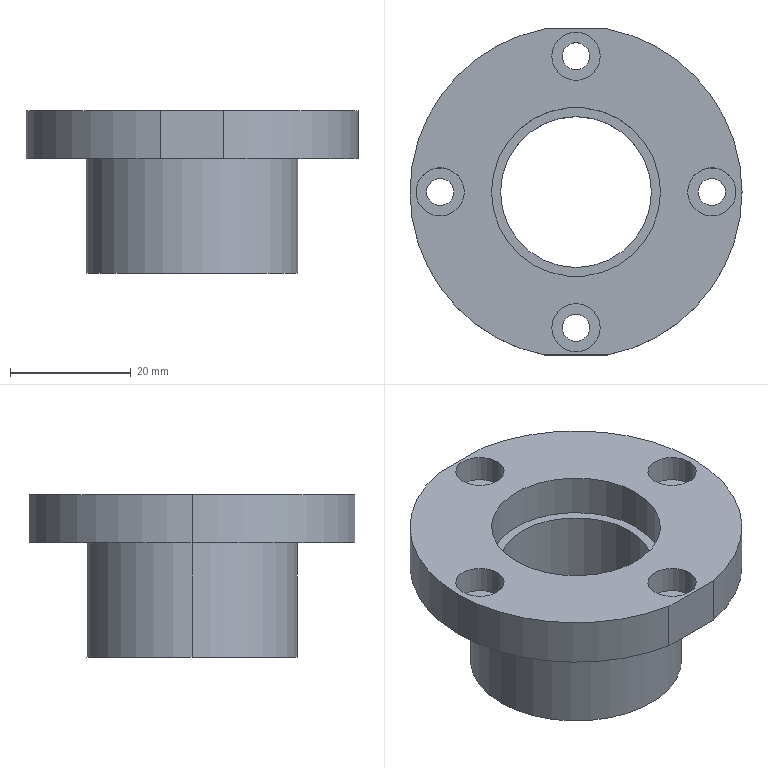Part | STEP file | 11-FG-E03611 | 1 solid | 38 faces | box 55 x 54 x 27 mm | volume 21102 mm3 | cylinder 27 | plane 11 | commonest cylinder face diameters 4.5 x8 8 x8 28 x4 55 x3 25 x2 35 x2
STEP:
#1=CARTESIAN_POINT('',(-26.5,0.,22.5));
#2=VERTEX_POINT('',#1);
#3=CARTESIAN_POINT('',(-18.5,0.,22.5));
#4=VERTEX_POINT('',#3);
#5=CARTESIAN_POINT('',(-22.5,0.,22.5));
#6=DIRECTION('',(0.,0.,1.));
#7=DIRECTION('',(1.,0.,0.));
#8=AXIS2_PLACEMENT_3D('',#5,#6,#7);
#9=CIRCLE('',#8,4.);
#10=EDGE_CURVE('',#2,#4,#9,.T.);
#11=ORIENTED_EDGE('',*,*,#10,.F.);
#12=CARTESIAN_POINT('',(-26.5,0.,27.));
#13=VERTEX_POINT('',#12);
#14=CARTESIAN_POINT('',(-26.5,0.,27.));
#15=DIRECTION('',(0.,0.,1.));
#16=VECTOR('',#15,1000.);
#17=LINE('',#14,#16);
#18=EDGE_CURVE('',#2,#13,#17,.T.);
#19=ORIENTED_EDGE('',*,*,#18,.T.);
#20=CARTESIAN_POINT('',(-18.5,0.,27.));
#21=VERTEX_POINT('',#20);
#22=CARTESIAN_POINT('',(-22.5,0.,27.));
#23=DIRECTION('',(0.,0.,1.));
#24=DIRECTION('',(1.,0.,0.));
#25=AXIS2_PLACEMENT_3D('',#22,#23,#24);
#26=CIRCLE('',#25,4.);
#27=EDGE_CURVE('',#13,#21,#26,.T.);
#28=ORIENTED_EDGE('',*,*,#27,.T.);
#29=CARTESIAN_POINT('',(-18.5,0.,27.));
#30=DIRECTION('',(0.,0.,1.));
#31=VECTOR('',#30,1000.);
#32=LINE('',#29,#31);
#33=EDGE_CURVE('',#4,#21,#32,.T.);
#34=ORIENTED_EDGE('',*,*,#33,.F.);
#35=EDGE_LOOP('',(#11,#19,#28,#34));
#36=FACE_OUTER_BOUND('',#35,.T.);
#37=CARTESIAN_POINT('',(-22.5,0.,27.));
#38=DIRECTION('',(0.,0.,1.));
#39=DIRECTION('',(1.,0.,0.));
#40=AXIS2_PLACEMENT_3D('',#37,#38,#39);
#41=CYLINDRICAL_SURFACE('',#40,4.);
#42=ADVANCED_FACE('',(#36),#41,.F.);
#43=CARTESIAN_POINT('',(-24.75,0.,19.));
#44=VERTEX_POINT('',#43);
#45=CARTESIAN_POINT('',(-20.25,0.,19.));
#46=VERTEX_POINT('',#45);
#47=CARTESIAN_POINT('',(-22.5,0.,19.));
#48=DIRECTION('',(0.,0.,1.));
#49=DIRECTION('',(1.,0.,0.));
#50=AXIS2_PLACEMENT_3D('',#47,#48,#49);
#51=CIRCLE('',#50,2.25);
#52=EDGE_CURVE('',#44,#46,#51,.T.);
#53=ORIENTED_EDGE('',*,*,#52,.F.);
#54=CARTESIAN_POINT('',(-24.75,0.,22.5));
#55=VERTEX_POINT('',#54);
#56=CARTESIAN_POINT('',(-24.75,0.,27.));
#57=DIRECTION('',(0.,0.,1.));
#58=VECTOR('',#57,1000.);
#59=LINE('',#56,#58);
#60=EDGE_CURVE('',#44,#55,#59,.T.);
#61=ORIENTED_EDGE('',*,*,#60,.T.);
#62=CARTESIAN_POINT('',(-20.25,0.,22.5));
#63=VERTEX_POINT('',#62);
#64=CARTESIAN_POINT('',(-22.5,0.,22.5));
#65=DIRECTION('',(0.,0.,1.));
#66=DIRECTION('',(1.,0.,0.));
#67=AXIS2_PLACEMENT_3D('',#64,#65,#66);
#68=CIRCLE('',#67,2.25);
#69=EDGE_CURVE('',#55,#63,#68,.T.);
#70=ORIENTED_EDGE('',*,*,#69,.T.);
#71=CARTESIAN_POINT('',(-20.25,0.,27.));
#72=DIRECTION('',(0.,0.,1.));
#73=VECTOR('',#72,1000.);
#74=LINE('',#71,#73);
#75=EDGE_CURVE('',#46,#63,#74,.T.);
#76=ORIENTED_EDGE('',*,*,#75,.F.);
#77=EDGE_LOOP('',(#53,#61,#70,#76));
#78=FACE_OUTER_BOUND('',#77,.T.);
#79=CARTESIAN_POINT('',(-22.5,0.,27.));
#80=DIRECTION('',(0.,0.,1.));
#81=DIRECTION('',(1.,0.,0.));
#82=AXIS2_PLACEMENT_3D('',#79,#80,#81);
#83=CYLINDRICAL_SURFACE('',#82,2.25);
#84=ADVANCED_FACE('',(#78),#83,.F.);
#85=CARTESIAN_POINT('',(-4.,-22.5,22.5));
#86=VERTEX_POINT('',#85);
#87=CARTESIAN_POINT('',(4.,-22.5,22.5));
#88=VERTEX_POINT('',#87);
#89=CARTESIAN_POINT('',(0.,-22.5,22.5));
#90=DIRECTION('',(0.,0.,1.));
#91=DIRECTION('',(1.,0.,0.));
#92=AXIS2_PLACEMENT_3D('',#89,#90,#91);
#93=CIRCLE('',#92,4.);
#94=EDGE_CURVE('',#86,#88,#93,.T.);
#95=ORIENTED_EDGE('',*,*,#94,.F.);
#96=CARTESIAN_POINT('',(-4.,-22.5,27.));
#97=VERTEX_POINT('',#96);
#98=CARTESIAN_POINT('',(-4.,-22.5,27.));
#99=DIRECTION('',(0.,0.,1.));
#100=VECTOR('',#99,1000.);
#101=LINE('',#98,#100);
#102=EDGE_CURVE('',#86,#97,#101,.T.);
#103=ORIENTED_EDGE('',*,*,#102,.T.);
#104=CARTESIAN_POINT('',(4.,-22.5,27.));
#105=VERTEX_POINT('',#104);
#106=CARTESIAN_POINT('',(0.,-22.5,27.));
#107=DIRECTION('',(0.,0.,1.));
#108=DIRECTION('',(1.,0.,0.));
#109=AXIS2_PLACEMENT_3D('',#106,#107,#108);
#110=CIRCLE('',#109,4.);
#111=EDGE_CURVE('',#97,#105,#110,.T.);
#112=ORIENTED_EDGE('',*,*,#111,.T.);
#113=CARTESIAN_POINT('',(4.,-22.5,27.));
#114=DIRECTION('',(0.,0.,1.));
#115=VECTOR('',#114,1000.);
#116=LINE('',#113,#115);
#117=EDGE_CURVE('',#88,#105,#116,.T.);
#118=ORIENTED_EDGE('',*,*,#117,.F.);
#119=EDGE_LOOP('',(#95,#103,#112,#118));
#120=FACE_OUTER_BOUND('',#119,.T.);
#121=CARTESIAN_POINT('',(0.,-22.5,27.));
#122=DIRECTION('',(0.,0.,1.));
#123=DIRECTION('',(1.,0.,0.));
#124=AXIS2_PLACEMENT_3D('',#121,#122,#123);
#125=CYLINDRICAL_SURFACE('',#124,4.);
#126=ADVANCED_FACE('',(#120),#125,.F.);
#127=CARTESIAN_POINT('',(-2.25,-22.5,19.));
#128=VERTEX_POINT('',#127);
#129=CARTESIAN_POINT('',(2.25,-22.5,19.));
#130=VERTEX_POINT('',#129);
#131=CARTESIAN_POINT('',(0.,-22.5,19.));
#132=DIRECTION('',(0.,0.,1.));
#133=DIRECTION('',(1.,0.,0.));
#134=AXIS2_PLACEMENT_3D('',#131,#132,#133);
#135=CIRCLE('',#134,2.25);
#136=EDGE_CURVE('',#128,#130,#135,.T.);
#137=ORIENTED_EDGE('',*,*,#136,.F.);
#138=CARTESIAN_POINT('',(-2.25,-22.5,22.5));
#139=VERTEX_POINT('',#138);
#140=CARTESIAN_POINT('',(-2.25,-22.5,27.));
#141=DIRECTION('',(0.,0.,1.));
#142=VECTOR('',#141,1000.);
#143=LINE('',#140,#142);
#144=EDGE_CURVE('',#128,#139,#143,.T.);
#145=ORIENTED_EDGE('',*,*,#144,.T.);
#146=CARTESIAN_POINT('',(2.25,-22.5,22.5));
#147=VERTEX_POINT('',#146);
#148=CARTESIAN_POINT('',(0.,-22.5,22.5));
#149=DIRECTION('',(0.,0.,1.));
#150=DIRECTION('',(1.,0.,0.));
#151=AXIS2_PLACEMENT_3D('',#148,#149,#150);
#152=CIRCLE('',#151,2.25);
#153=EDGE_CURVE('',#139,#147,#152,.T.);
#154=ORIENTED_EDGE('',*,*,#153,.T.);
#155=CARTESIAN_POINT('',(2.25,-22.5,27.));
#156=DIRECTION('',(0.,0.,1.));
#157=VECTOR('',#156,1000.);
#158=LINE('',#155,#157);
#159=EDGE_CURVE('',#130,#147,#158,.T.);
#160=ORIENTED_EDGE('',*,*,#159,.F.);
#161=EDGE_LOOP('',(#137,#145,#154,#160));
#162=FACE_OUTER_BOUND('',#161,.T.);
#163=CARTESIAN_POINT('',(0.,-22.5,27.));
#164=DIRECTION('',(0.,0.,1.));
#165=DIRECTION('',(1.,0.,0.));
#166=AXIS2_PLACEMENT_3D('',#163,#164,#165);
#167=CYLINDRICAL_SURFACE('',#166,2.25);
#168=ADVANCED_FACE('',(#162),#167,.F.);
#169=CARTESIAN_POINT('',(18.5,0.,22.5));
#170=VERTEX_POINT('',#169);
#171=CARTESIAN_POINT('',(26.5,0.,22.5));
#172=VERTEX_POINT('',#171);
#173=CARTESIAN_POINT('',(22.5,0.,22.5));
#174=DIRECTION('',(0.,0.,1.));
#175=DIRECTION('',(1.,0.,0.));
#176=AXIS2_PLACEMENT_3D('',#173,#174,#175);
#177=CIRCLE('',#176,4.);
#178=EDGE_CURVE('',#170,#172,#177,.T.);
#179=ORIENTED_EDGE('',*,*,#178,.F.);
#180=CARTESIAN_POINT('',(18.5,0.,27.));
#181=VERTEX_POINT('',#180);
#182=CARTESIAN_POINT('',(18.5,0.,27.));
#183=DIRECTION('',(0.,0.,1.));
#184=VECTOR('',#183,1000.);
#185=LINE('',#182,#184);
#186=EDGE_CURVE('',#170,#181,#185,.T.);
#187=ORIENTED_EDGE('',*,*,#186,.T.);
#188=CARTESIAN_POINT('',(26.5,0.,27.));
#189=VERTEX_POINT('',#188);
#190=CARTESIAN_POINT('',(22.5,0.,27.));
#191=DIRECTION('',(0.,0.,1.));
#192=DIRECTION('',(1.,0.,0.));
#193=AXIS2_PLACEMENT_3D('',#190,#191,#192);
#194=CIRCLE('',#193,4.);
#195=EDGE_CURVE('',#181,#189,#194,.T.);
#196=ORIENTED_EDGE('',*,*,#195,.T.);
#197=CARTESIAN_POINT('',(26.5,0.,27.));
#198=DIRECTION('',(0.,0.,1.));
#199=VECTOR('',#198,1000.);
#200=LINE('',#197,#199);
#201=EDGE_CURVE('',#172,#189,#200,.T.);
#202=ORIENTED_EDGE('',*,*,#201,.F.);
#203=EDGE_LOOP('',(#179,#187,#196,#202));
#204=FACE_OUTER_BOUND('',#203,.T.);
#205=CARTESIAN_POINT('',(22.5,0.,27.));
#206=DIRECTION('',(0.,0.,1.));
#207=DIRECTION('',(1.,0.,0.));
#208=AXIS2_PLACEMENT_3D('',#205,#206,#207);
#209=CYLINDRICAL_SURFACE('',#208,4.);
#210=ADVANCED_FACE('',(#204),#209,.F.);
#211=CARTESIAN_POINT('',(20.25,0.,19.));
#212=VERTEX_POINT('',#211);
#213=CARTESIAN_POINT('',(24.75,0.,19.));
#214=VERTEX_POINT('',#213);
#215=CARTESIAN_POINT('',(22.5,0.,19.));
#216=DIRECTION('',(0.,0.,1.));
#217=DIRECTION('',(1.,0.,0.));
#218=AXIS2_PLACEMENT_3D('',#215,#216,#217);
#219=CIRCLE('',#218,2.25);
#220=EDGE_CURVE('',#212,#214,#219,.T.);
#221=ORIENTED_EDGE('',*,*,#220,.F.);
#222=CARTESIAN_POINT('',(20.25,0.,22.5));
#223=VERTEX_POINT('',#222);
#224=CARTESIAN_POINT('',(20.25,0.,27.));
#225=DIRECTION('',(0.,0.,1.));
#226=VECTOR('',#225,1000.);
#227=LINE('',#224,#226);
#228=EDGE_CURVE('',#212,#223,#227,.T.);
#229=ORIENTED_EDGE('',*,*,#228,.T.);
#230=CARTESIAN_POINT('',(24.75,0.,22.5));
#231=VERTEX_POINT('',#230);
#232=CARTESIAN_POINT('',(22.5,0.,22.5));
#233=DIRECTION('',(0.,0.,1.));
#234=DIRECTION('',(1.,0.,0.));
#235=AXIS2_PLACEMENT_3D('',#232,#233,#234);
#236=CIRCLE('',#235,2.25);
#237=EDGE_CURVE('',#223,#231,#236,.T.);
#238=ORIENTED_EDGE('',*,*,#237,.T.);
#239=CARTESIAN_POINT('',(24.75,0.,27.));
#240=DIRECTION('',(0.,0.,1.));
#241=VECTOR('',#240,1000.);
#242=LINE('',#239,#241);
#243=EDGE_CURVE('',#214,#231,#242,.T.);
#244=ORIENTED_EDGE('',*,*,#243,.F.);
#245=EDGE_LOOP('',(#221,#229,#238,#244));
#246=FACE_OUTER_BOUND('',#245,.T.);
#247=CARTESIAN_POINT('',(22.5,0.,27.));
#248=DIRECTION('',(0.,0.,1.));
#249=DIRECTION('',(1.,0.,0.));
#250=AXIS2_PLACEMENT_3D('',#247,#248,#249);
#251=CYLINDRICAL_SURFACE('',#250,2.25);
#252=ADVANCED_FACE('',(#246),#251,.F.);
#253=CARTESIAN_POINT('',(-4.,22.5,22.5));
#254=VERTEX_POINT('',#253);
#255=CARTESIAN_POINT('',(4.,22.5,22.5));
#256=VERTEX_POINT('',#255);
#257=CARTESIAN_POINT('',(0.,22.5,22.5));
#258=DIRECTION('',(0.,0.,1.));
#259=DIRECTION('',(1.,0.,0.));
#260=AXIS2_PLACEMENT_3D('',#257,#258,#259);
#261=CIRCLE('',#260,4.);
#262=EDGE_CURVE('',#254,#256,#261,.T.);
#263=ORIENTED_EDGE('',*,*,#262,.F.);
#264=CARTESIAN_POINT('',(-4.,22.5,27.));
#265=VERTEX_POINT('',#264);
#266=CARTESIAN_POINT('',(-4.,22.5,27.));
#267=DIRECTION('',(0.,0.,1.));
#268=VECTOR('',#267,1000.);
#269=LINE('',#266,#268);
#270=EDGE_CURVE('',#254,#265,#269,.T.);
#271=ORIENTED_EDGE('',*,*,#270,.T.);
#272=CARTESIAN_POINT('',(4.,22.5,27.));
#273=VERTEX_POINT('',#272);
#274=CARTESIAN_POINT('',(0.,22.5,27.));
#275=DIRECTION('',(0.,0.,1.));
#276=DIRECTION('',(1.,0.,0.));
#277=AXIS2_PLACEMENT_3D('',#274,#275,#276);
#278=CIRCLE('',#277,4.);
#279=EDGE_CURVE('',#265,#273,#278,.T.);
#280=ORIENTED_EDGE('',*,*,#279,.T.);
#281=CARTESIAN_POINT('',(4.,22.5,27.));
#282=DIRECTION('',(0.,0.,1.));
#283=VECTOR('',#282,1000.);
#284=LINE('',#281,#283);
#285=EDGE_CURVE('',#256,#273,#284,.T.);
#286=ORIENTED_EDGE('',*,*,#285,.F.);
#287=EDGE_LOOP('',(#263,#271,#280,#286));
#288=FACE_OUTER_BOUND('',#287,.T.);
#289=CARTESIAN_POINT('',(0.,22.5,27.));
#290=DIRECTION('',(0.,0.,1.));
#291=DIRECTION('',(1.,0.,0.));
#292=AXIS2_PLACEMENT_3D('',#289,#290,#291);
#293=CYLINDRICAL_SURFACE('',#292,4.);
#294=ADVANCED_FACE('',(#288),#293,.F.);
#295=CARTESIAN_POINT('',(-2.25,22.5,19.));
#296=VERTEX_POINT('',#295);
#297=CARTESIAN_POINT('',(2.25,22.5,19.));
#298=VERTEX_POINT('',#297);
#299=CARTESIAN_POINT('',(0.,22.5,19.));
#300=DIRECTION('',(0.,0.,1.));
#301=DIRECTION('',(1.,0.,0.));
#302=AXIS2_PLACEMENT_3D('',#299,#300,#301);
#303=CIRCLE('',#302,2.25);
#304=EDGE_CURVE('',#296,#298,#303,.T.);
#305=ORIENTED_EDGE('',*,*,#304,.F.);
#306=CARTESIAN_POINT('',(-2.25,22.5,22.5));
#307=VERTEX_POINT('',#306);
#308=CARTESIAN_POINT('',(-2.25,22.5,27.));
#309=DIRECTION('',(0.,0.,1.));
#310=VECTOR('',#309,1000.);
#311=LINE('',#308,#310);
#312=EDGE_CURVE('',#296,#307,#311,.T.);
#313=ORIENTED_EDGE('',*,*,#312,.T.);
#314=CARTESIAN_POINT('',(2.25,22.5,22.5));
#315=VERTEX_POINT('',#314);
#316=CARTESIAN_POINT('',(0.,22.5,22.5));
#317=DIRECTION('',(0.,0.,1.));
#318=DIRECTION('',(1.,0.,0.));
#319=AXIS2_PLACEMENT_3D('',#316,#317,#318);
#320=CIRCLE('',#319,2.25);
#321=EDGE_CURVE('',#307,#315,#320,.T.);
#322=ORIENTED_EDGE('',*,*,#321,.T.);
#323=CARTESIAN_POINT('',(2.25,22.5,27.));
#324=DIRECTION('',(0.,0.,1.));
#325=VECTOR('',#324,1000.);
#326=LINE('',#323,#325);
#327=EDGE_CURVE('',#298,#315,#326,.T.);
#328=ORIENTED_EDGE('',*,*,#327,.F.);
#329=EDGE_LOOP('',(#305,#313,#322,#328));
#330=FACE_OUTER_BOUND('',#329,.T.);
#331=CARTESIAN_POINT('',(0.,22.5,27.));
#332=DIRECTION('',(0.,0.,1.));
#333=DIRECTION('',(1.,0.,0.));
#334=AXIS2_PLACEMENT_3D('',#331,#332,#333);
#335=CYLINDRICAL_SURFACE('',#334,2.25);
#336=ADVANCED_FACE('',(#330),#335,.F.);
#337=CARTESIAN_POINT('',(-14.,0.,20.));
#338=VERTEX_POINT('',#337);
#339=CARTESIAN_POINT('',(14.,0.,20.));
#340=VERTEX_POINT('',#339);
#341=CARTESIAN_POINT('',(0.,0.,20.));
#342=DIRECTION('',(0.,0.,1.));
#343=DIRECTION('',(1.,0.,0.));
#344=AXIS2_PLACEMENT_3D('',#341,#342,#343);
#345=CIRCLE('',#344,14.);
#346=EDGE_CURVE('',#338,#340,#345,.T.);
#347=ORIENTED_EDGE('',*,*,#346,.F.);
#348=CARTESIAN_POINT('',(-14.,0.,27.));
#349=VERTEX_POINT('',#348);
#350=CARTESIAN_POINT('',(-14.,0.,20.));
#351=DIRECTION('',(0.,0.,1.));
#352=VECTOR('',#351,1000.);
#353=LINE('',#350,#352);
#354=EDGE_CURVE('',#338,#349,#353,.T.);
#355=ORIENTED_EDGE('',*,*,#354,.T.);
#356=CARTESIAN_POINT('',(14.,0.,27.));
#357=VERTEX_POINT('',#356);
#358=CARTESIAN_POINT('',(0.,0.,27.));
#359=DIRECTION('',(0.,0.,1.));
#360=DIRECTION('',(1.,0.,0.));
#361=AXIS2_PLACEMENT_3D('',#358,#359,#360);
#362=CIRCLE('',#361,14.);
#363=EDGE_CURVE('',#349,#357,#362,.T.);
#364=ORIENTED_EDGE('',*,*,#363,.T.);
#365=CARTESIAN_POINT('',(14.,0.,20.));
#366=DIRECTION('',(0.,0.,1.));
#367=VECTOR('',#366,1000.);
#368=LINE('',#365,#367);
#369=EDGE_CURVE('',#340,#357,#368,.T.);
#370=ORIENTED_EDGE('',*,*,#369,.F.);
#371=EDGE_LOOP('',(#347,#355,#364,#370));
#372=FACE_OUTER_BOUND('',#371,.T.);
#373=CARTESIAN_POINT('',(0.,0.,20.));
#374=DIRECTION('',(0.,0.,1.));
#375=DIRECTION('',(1.,0.,0.));
#376=AXIS2_PLACEMENT_3D('',#373,#374,#375);
#377=CYLINDRICAL_SURFACE('',#376,14.);
#378=ADVANCED_FACE('',(#372),#377,.F.);
#379=CARTESIAN_POINT('',(14.,0.,7.));
#380=VERTEX_POINT('',#379);
#381=CARTESIAN_POINT('',(-14.,0.,7.));
#382=VERTEX_POINT('',#381);
#383=CARTESIAN_POINT('',(0.,0.,7.));
#384=DIRECTION('',(0.,0.,-1.));
#385=DIRECTION('',(-1.,0.,0.));
#386=AXIS2_PLACEMENT_3D('',#383,#384,#385);
#387=CIRCLE('',#386,14.);
#388=EDGE_CURVE('',#380,#382,#387,.T.);
#389=ORIENTED_EDGE('',*,*,#388,.F.);
#390=CARTESIAN_POINT('',(14.,0.,0.));
#391=VERTEX_POINT('',#390);
#392=CARTESIAN_POINT('',(14.,0.,7.));
#393=DIRECTION('',(0.,0.,-1.));
#394=VECTOR('',#393,1000.);
#395=LINE('',#392,#394);
#396=EDGE_CURVE('',#380,#391,#395,.T.);
#397=ORIENTED_EDGE('',*,*,#396,.T.);
#398=CARTESIAN_POINT('',(-14.,0.,0.));
#399=VERTEX_POINT('',#398);
#400=CARTESIAN_POINT('',(0.,0.,0.));
#401=DIRECTION('',(0.,0.,-1.));
#402=DIRECTION('',(-1.,0.,0.));
#403=AXIS2_PLACEMENT_3D('',#400,#401,#402);
#404=CIRCLE('',#403,14.);
#405=EDGE_CURVE('',#391,#399,#404,.T.);
#406=ORIENTED_EDGE('',*,*,#405,.T.);
#407=CARTESIAN_POINT('',(-14.,0.,7.));
#408=DIRECTION('',(0.,0.,-1.));
#409=VECTOR('',#408,1000.);
#410=LINE('',#407,#409);
#411=EDGE_CURVE('',#382,#399,#410,.T.);
#412=ORIENTED_EDGE('',*,*,#411,.F.);
#413=EDGE_LOOP('',(#389,#397,#406,#412));
#414=FACE_OUTER_BOUND('',#413,.T.);
#415=CARTESIAN_POINT('',(0.,0.,7.));
#416=DIRECTION('',(0.,0.,-1.));
#417=DIRECTION('',(-1.,0.,0.));
#418=AXIS2_PLACEMENT_3D('',#415,#416,#417);
#419=CYLINDRICAL_SURFACE('',#418,14.);
#420=ADVANCED_FACE('',(#414),#419,.F.);
#421=CARTESIAN_POINT('',(-27.5,0.,27.));
#422=VERTEX_POINT('',#421);
#423=CARTESIAN_POINT('',(-5.22,-27.,27.));
#424=VERTEX_POINT('',#423);
#425=CARTESIAN_POINT('',(0.,0.,27.));
#426=DIRECTION('',(0.,0.,1.));
#427=DIRECTION('',(1.,0.,0.));
#428=AXIS2_PLACEMENT_3D('',#425,#426,#427);
#429=CIRCLE('',#428,27.5);
#430=EDGE_CURVE('',#422,#424,#429,.T.);
#431=ORIENTED_EDGE('',*,*,#430,.F.);
#432=CARTESIAN_POINT('',(-27.5,0.,19.));
#433=VERTEX_POINT('',#432);
#434=CARTESIAN_POINT('',(-27.5,0.,27.));
#435=DIRECTION('',(0.,0.,-1.));
#436=VECTOR('',#435,1000.);
#437=LINE('',#434,#436);
#438=EDGE_CURVE('',#422,#433,#437,.T.);
#439=ORIENTED_EDGE('',*,*,#438,.T.);
#440=CARTESIAN_POINT('',(-5.22,-27.,19.));
#441=VERTEX_POINT('',#440);
#442=CARTESIAN_POINT('',(0.,0.,19.));
#443=DIRECTION('',(0.,0.,1.));
#444=DIRECTION('',(1.,0.,0.));
#445=AXIS2_PLACEMENT_3D('',#442,#443,#444);
#446=CIRCLE('',#445,27.5);
#447=EDGE_CURVE('',#433,#441,#446,.T.);
#448=ORIENTED_EDGE('',*,*,#447,.T.);
#449=CARTESIAN_POINT('',(-5.22,-27.,27.));
#450=DIRECTION('',(0.,0.,1.));
#451=VECTOR('',#450,1000.);
#452=LINE('',#449,#451);
#453=EDGE_CURVE('',#441,#424,#452,.T.);
#454=ORIENTED_EDGE('',*,*,#453,.T.);
#455=EDGE_LOOP('',(#431,#439,#448,#454));
#456=FACE_OUTER_BOUND('',#455,.T.);
#457=CARTESIAN_POINT('',(0.,0.,27.));
#458=DIRECTION('',(0.,0.,-1.));
#459=DIRECTION('',(-1.,0.,0.));
#460=AXIS2_PLACEMENT_3D('',#457,#458,#459);
#461=CYLINDRICAL_SURFACE('',#460,27.5);
#462=ADVANCED_FACE('',(#456),#461,.T.);
#463=CARTESIAN_POINT('',(17.5,0.,19.));
#464=VERTEX_POINT('',#463);
#465=CARTESIAN_POINT('',(-17.5,0.,19.));
#466=VERTEX_POINT('',#465);
#467=CARTESIAN_POINT('',(0.,0.,19.));
#468=DIRECTION('',(0.,0.,1.));
#469=DIRECTION('',(1.,0.,0.));
#470=AXIS2_PLACEMENT_3D('',#467,#468,#469);
#471=CIRCLE('',#470,17.5);
#472=EDGE_CURVE('',#464,#466,#471,.T.);
#473=ORIENTED_EDGE('',*,*,#472,.F.);
#474=CARTESIAN_POINT('',(17.5,0.,0.));
#475=VERTEX_POINT('',#474);
#476=CARTESIAN_POINT('',(17.5,0.,19.));
#477=DIRECTION('',(0.,0.,-1.));
#478=VECTOR('',#477,1000.);
#479=LINE('',#476,#478);
#480=EDGE_CURVE('',#464,#475,#479,.T.);
#481=ORIENTED_EDGE('',*,*,#480,.T.);
#482=CARTESIAN_POINT('',(-17.5,0.,0.));
#483=VERTEX_POINT('',#482);
#484=CARTESIAN_POINT('',(0.,0.,0.));
#485=DIRECTION('',(0.,0.,1.));
#486=DIRECTION('',(1.,0.,0.));
#487=AXIS2_PLACEMENT_3D('',#484,#485,#486);
#488=CIRCLE('',#487,17.5);
#489=EDGE_CURVE('',#475,#483,#488,.T.);
#490=ORIENTED_EDGE('',*,*,#489,.T.);
#491=CARTESIAN_POINT('',(-17.5,0.,19.));
#492=DIRECTION('',(0.,0.,-1.));
#493=VECTOR('',#492,1000.);
#494=LINE('',#491,#493);
#495=EDGE_CURVE('',#466,#483,#494,.T.);
#496=ORIENTED_EDGE('',*,*,#495,.F.);
#497=EDGE_LOOP('',(#473,#481,#490,#496));
#498=FACE_OUTER_BOUND('',#497,.T.);
#499=CARTESIAN_POINT('',(0.,0.,19.));
#500=DIRECTION('',(0.,0.,-1.));
#501=DIRECTION('',(-1.,0.,0.));
#502=AXIS2_PLACEMENT_3D('',#499,#500,#501);
#503=CYLINDRICAL_SURFACE('',#502,17.5);
#504=ADVANCED_FACE('',(#498),#503,.T.);
#505=CARTESIAN_POINT('',(-12.5,0.,20.));
#506=VERTEX_POINT('',#505);
#507=CARTESIAN_POINT('',(12.5,0.,20.));
#508=VERTEX_POINT('',#507);
#509=CARTESIAN_POINT('',(0.,0.,20.));
#510=DIRECTION('',(0.,0.,1.));
#511=DIRECTION('',(1.,0.,0.));
#512=AXIS2_PLACEMENT_3D('',#509,#510,#511);
#513=CIRCLE('',#512,12.5);
#514=EDGE_CURVE('',#506,#508,#513,.T.);
#515=ORIENTED_EDGE('',*,*,#514,.T.);
#516=CARTESIAN_POINT('',(12.5,0.,7.));
#517=VERTEX_POINT('',#516);
#518=CARTESIAN_POINT('',(12.5,0.,27.));
#519=DIRECTION('',(0.,0.,-1.));
#520=VECTOR('',#519,1000.);
#521=LINE('',#518,#520);
#522=EDGE_CURVE('',#508,#517,#521,.T.);
#523=ORIENTED_EDGE('',*,*,#522,.T.);
#524=CARTESIAN_POINT('',(-12.5,0.,7.));
#525=VERTEX_POINT('',#524);
#526=CARTESIAN_POINT('',(0.,0.,7.));
#527=DIRECTION('',(0.,0.,-1.));
#528=DIRECTION('',(-1.,0.,0.));
#529=AXIS2_PLACEMENT_3D('',#526,#527,#528);
#530=CIRCLE('',#529,12.5);
#531=EDGE_CURVE('',#517,#525,#530,.T.);
#532=ORIENTED_EDGE('',*,*,#531,.T.);
#533=CARTESIAN_POINT('',(-12.5,0.,27.));
#534=DIRECTION('',(0.,0.,-1.));
#535=VECTOR('',#534,1000.);
#536=LINE('',#533,#535);
#537=EDGE_CURVE('',#506,#525,#536,.T.);
#538=ORIENTED_EDGE('',*,*,#537,.F.);
#539=EDGE_LOOP('',(#515,#523,#532,#538));
#540=FACE_OUTER_BOUND('',#539,.T.);
#541=CARTESIAN_POINT('',(0.,0.,27.));
#542=DIRECTION('',(0.,0.,-1.));
#543=DIRECTION('',(-1.,0.,0.));
#544=AXIS2_PLACEMENT_3D('',#541,#542,#543);
#545=CYLINDRICAL_SURFACE('',#544,12.5);
#546=ADVANCED_FACE('',(#540),#545,.F.);
#547=CARTESIAN_POINT('',(5.22,-27.,27.));
#548=VERTEX_POINT('',#547);
#549=CARTESIAN_POINT('',(5.22,27.,27.));
#550=VERTEX_POINT('',#549);
#551=CARTESIAN_POINT('',(0.,0.,27.));
#552=DIRECTION('',(0.,0.,1.));
#553=DIRECTION('',(1.,0.,0.));
#554=AXIS2_PLACEMENT_3D('',#551,#552,#553);
#555=CIRCLE('',#554,27.5);
#556=EDGE_CURVE('',#548,#550,#555,.T.);
#557=ORIENTED_EDGE('',*,*,#556,.F.);
#558=CARTESIAN_POINT('',(5.22,-27.,19.));
#559=VERTEX_POINT('',#558);
#560=CARTESIAN_POINT('',(5.22,-27.,27.));
#561=DIRECTION('',(0.,0.,-1.));
#562=VECTOR('',#561,1000.);
#563=LINE('',#560,#562);
#564=EDGE_CURVE('',#548,#559,#563,.T.);
#565=ORIENTED_EDGE('',*,*,#564,.T.);
#566=CARTESIAN_POINT('',(5.22,27.,19.));
#567=VERTEX_POINT('',#566);
#568=CARTESIAN_POINT('',(0.,0.,19.));
#569=DIRECTION('',(0.,0.,1.));
#570=DIRECTION('',(1.,0.,0.));
#571=AXIS2_PLACEMENT_3D('',#568,#569,#570);
#572=CIRCLE('',#571,27.5);
#573=EDGE_CURVE('',#559,#567,#572,.T.);
#574=ORIENTED_EDGE('',*,*,#573,.T.);
#575=CARTESIAN_POINT('',(5.22,27.,27.));
#576=DIRECTION('',(0.,0.,1.));
#577=VECTOR('',#576,1000.);
#578=LINE('',#575,#577);
#579=EDGE_CURVE('',#567,#550,#578,.T.);
#580=ORIENTED_EDGE('',*,*,#579,.T.);
#581=EDGE_LOOP('',(#557,#565,#574,#580));
#582=FACE_OUTER_BOUND('',#581,.T.);
#583=CARTESIAN_POINT('',(0.,0.,27.));
#584=DIRECTION('',(0.,0.,-1.));
#585=DIRECTION('',(-1.,0.,0.));
#586=AXIS2_PLACEMENT_3D('',#583,#584,#585);
#587=CYLINDRICAL_SURFACE('',#586,27.5);
#588=ADVANCED_FACE('',(#582),#587,.T.);
#589=ORIENTED_EDGE('',*,*,#522,.F.);
#590=CARTESIAN_POINT('',(0.,0.,20.));
#591=DIRECTION('',(0.,0.,1.));
#592=DIRECTION('',(1.,0.,0.));
#593=AXIS2_PLACEMENT_3D('',#590,#591,#592);
#594=CIRCLE('',#593,12.5);
#595=EDGE_CURVE('',#508,#506,#594,.T.);
#596=ORIENTED_EDGE('',*,*,#595,.T.);
#597=ORIENTED_EDGE('',*,*,#537,.T.);
#598=CARTESIAN_POINT('',(0.,0.,7.));
#599=DIRECTION('',(0.,0.,-1.));
#600=DIRECTION('',(-1.,0.,0.));
#601=AXIS2_PLACEMENT_3D('',#598,#599,#600);
#602=CIRCLE('',#601,12.5);
#603=EDGE_CURVE('',#525,#517,#602,.T.);
#604=ORIENTED_EDGE('',*,*,#603,.T.);
#605=EDGE_LOOP('',(#589,#596,#597,#604));
#606=FACE_OUTER_BOUND('',#605,.T.);
#607=CARTESIAN_POINT('',(0.,0.,27.));
#608=DIRECTION('',(0.,0.,-1.));
#609=DIRECTION('',(-1.,0.,0.));
#610=AXIS2_PLACEMENT_3D('',#607,#608,#609);
#611=CYLINDRICAL_SURFACE('',#610,12.5);
#612=ADVANCED_FACE('',(#606),#611,.F.);
#613=CARTESIAN_POINT('',(0.,0.,0.));
#614=DIRECTION('',(0.,0.,-1.));
#615=DIRECTION('',(-1.,0.,0.));
#616=AXIS2_PLACEMENT_3D('',#613,#614,#615);
#617=CIRCLE('',#616,14.);
#618=EDGE_CURVE('',#399,#391,#617,.T.);
#619=ORIENTED_EDGE('',*,*,#618,.F.);
#620=ORIENTED_EDGE('',*,*,#405,.F.);
#621=EDGE_LOOP('',(#619,#620));
#622=FACE_BOUND('',#621,.T.);
#623=CARTESIAN_POINT('',(0.,0.,0.));
#624=DIRECTION('',(0.,0.,1.));
#625=DIRECTION('',(1.,0.,0.));
#626=AXIS2_PLACEMENT_3D('',#623,#624,#625);
#627=CIRCLE('',#626,17.5);
#628=EDGE_CURVE('',#483,#475,#627,.T.);
#629=ORIENTED_EDGE('',*,*,#628,.F.);
#630=ORIENTED_EDGE('',*,*,#489,.F.);
#631=EDGE_LOOP('',(#629,#630));
#632=FACE_OUTER_BOUND('',#631,.T.);
#633=CARTESIAN_POINT('',(0.,0.,0.));
#634=DIRECTION('',(0.,0.,1.));
#635=DIRECTION('',(1.,0.,0.));
#636=AXIS2_PLACEMENT_3D('',#633,#634,#635);
#637=PLANE('',#636);
#638=ADVANCED_FACE('',(#622,#632),#637,.F.);
#639=CARTESIAN_POINT('',(-5.22,-27.,27.));
#640=DIRECTION('',(-1.,0.,0.));
#641=VECTOR('',#640,1000.);
#642=LINE('',#639,#641);
#643=EDGE_CURVE('',#548,#424,#642,.T.);
#644=ORIENTED_EDGE('',*,*,#643,.F.);
#645=ORIENTED_EDGE('',*,*,#556,.T.);
#646=CARTESIAN_POINT('',(-5.22,27.,27.));
#647=VERTEX_POINT('',#646);
#648=CARTESIAN_POINT('',(-5.22,27.,27.));
#649=DIRECTION('',(1.,0.,0.));
#650=VECTOR('',#649,1000.);
#651=LINE('',#648,#650);
#652=EDGE_CURVE('',#647,#550,#651,.T.);
#653=ORIENTED_EDGE('',*,*,#652,.F.);
#654=CARTESIAN_POINT('',(0.,0.,27.));
#655=DIRECTION('',(0.,0.,1.));
#656=DIRECTION('',(1.,0.,0.));
#657=AXIS2_PLACEMENT_3D('',#654,#655,#656);
#658=CIRCLE('',#657,27.5);
#659=EDGE_CURVE('',#647,#422,#658,.T.);
#660=ORIENTED_EDGE('',*,*,#659,.T.);
#661=ORIENTED_EDGE('',*,*,#430,.T.);
#662=EDGE_LOOP('',(#644,#645,#653,#660,#661));
#663=FACE_OUTER_BOUND('',#662,.T.);
#664=CARTESIAN_POINT('',(-22.5,0.,27.));
#665=DIRECTION('',(0.,0.,1.));
#666=DIRECTION('',(1.,0.,0.));
#667=AXIS2_PLACEMENT_3D('',#664,#665,#666);
#668=CIRCLE('',#667,4.);
#669=EDGE_CURVE('',#21,#13,#668,.T.);
#670=ORIENTED_EDGE('',*,*,#669,.F.);
#671=ORIENTED_EDGE('',*,*,#27,.F.);
#672=EDGE_LOOP('',(#670,#671));
#673=FACE_BOUND('',#672,.T.);
#674=CARTESIAN_POINT('',(0.,-22.5,27.));
#675=DIRECTION('',(0.,0.,1.));
#676=DIRECTION('',(1.,0.,0.));
#677=AXIS2_PLACEMENT_3D('',#674,#675,#676);
#678=CIRCLE('',#677,4.);
#679=EDGE_CURVE('',#105,#97,#678,.T.);
#680=ORIENTED_EDGE('',*,*,#679,.F.);
#681=ORIENTED_EDGE('',*,*,#111,.F.);
#682=EDGE_LOOP('',(#680,#681));
#683=FACE_BOUND('',#682,.T.);
#684=CARTESIAN_POINT('',(22.5,0.,27.));
#685=DIRECTION('',(0.,0.,1.));
#686=DIRECTION('',(1.,0.,0.));
#687=AXIS2_PLACEMENT_3D('',#684,#685,#686);
#688=CIRCLE('',#687,4.);
#689=EDGE_CURVE('',#189,#181,#688,.T.);
#690=ORIENTED_EDGE('',*,*,#689,.F.);
#691=ORIENTED_EDGE('',*,*,#195,.F.);
#692=EDGE_LOOP('',(#690,#691));
#693=FACE_BOUND('',#692,.T.);
#694=CARTESIAN_POINT('',(0.,22.5,27.));
#695=DIRECTION('',(0.,0.,1.));
#696=DIRECTION('',(1.,0.,0.));
#697=AXIS2_PLACEMENT_3D('',#694,#695,#696);
#698=CIRCLE('',#697,4.);
#699=EDGE_CURVE('',#273,#265,#698,.T.);
#700=ORIENTED_EDGE('',*,*,#699,.F.);
#701=ORIENTED_EDGE('',*,*,#279,.F.);
#702=EDGE_LOOP('',(#700,#701));
#703=FACE_BOUND('',#702,.T.);
#704=CARTESIAN_POINT('',(0.,0.,27.));
#705=DIRECTION('',(0.,0.,1.));
#706=DIRECTION('',(1.,0.,0.));
#707=AXIS2_PLACEMENT_3D('',#704,#705,#706);
#708=CIRCLE('',#707,14.);
#709=EDGE_CURVE('',#357,#349,#708,.T.);
#710=ORIENTED_EDGE('',*,*,#709,.F.);
#711=ORIENTED_EDGE('',*,*,#363,.F.);
#712=EDGE_LOOP('',(#710,#711));
#713=FACE_BOUND('',#712,.T.);
#714=CARTESIAN_POINT('',(0.,0.,27.));
#715=DIRECTION('',(0.,0.,1.));
#716=DIRECTION('',(1.,0.,0.));
#717=AXIS2_PLACEMENT_3D('',#714,#715,#716);
#718=PLANE('',#717);
#719=ADVANCED_FACE('',(#663,#673,#683,#693,#703,#713),#718,.T.);
#720=ORIENTED_EDGE('',*,*,#480,.F.);
#721=CARTESIAN_POINT('',(0.,0.,19.));
#722=DIRECTION('',(0.,0.,1.));
#723=DIRECTION('',(1.,0.,0.));
#724=AXIS2_PLACEMENT_3D('',#721,#722,#723);
#725=CIRCLE('',#724,17.5);
#726=EDGE_CURVE('',#466,#464,#725,.T.);
#727=ORIENTED_EDGE('',*,*,#726,.F.);
#728=ORIENTED_EDGE('',*,*,#495,.T.);
#729=ORIENTED_EDGE('',*,*,#628,.T.);
#730=EDGE_LOOP('',(#720,#727,#728,#729));
#731=FACE_OUTER_BOUND('',#730,.T.);
#732=CARTESIAN_POINT('',(0.,0.,19.));
#733=DIRECTION('',(0.,0.,-1.));
#734=DIRECTION('',(-1.,0.,0.));
#735=AXIS2_PLACEMENT_3D('',#732,#733,#734);
#736=CYLINDRICAL_SURFACE('',#735,17.5);
#737=ADVANCED_FACE('',(#731),#736,.T.);
#738=CARTESIAN_POINT('',(-22.5,0.,19.));
#739=DIRECTION('',(0.,0.,1.));
#740=DIRECTION('',(1.,0.,0.));
#741=AXIS2_PLACEMENT_3D('',#738,#739,#740);
#742=CIRCLE('',#741,2.25);
#743=EDGE_CURVE('',#46,#44,#742,.T.);
#744=ORIENTED_EDGE('',*,*,#743,.T.);
#745=ORIENTED_EDGE('',*,*,#52,.T.);
#746=EDGE_LOOP('',(#744,#745));
#747=FACE_BOUND('',#746,.T.);
#748=CARTESIAN_POINT('',(0.,-22.5,19.));
#749=DIRECTION('',(0.,0.,1.));
#750=DIRECTION('',(1.,0.,0.));
#751=AXIS2_PLACEMENT_3D('',#748,#749,#750);
#752=CIRCLE('',#751,2.25);
#753=EDGE_CURVE('',#130,#128,#752,.T.);
#754=ORIENTED_EDGE('',*,*,#753,.T.);
#755=ORIENTED_EDGE('',*,*,#136,.T.);
#756=EDGE_LOOP('',(#754,#755));
#757=FACE_BOUND('',#756,.T.);
#758=CARTESIAN_POINT('',(22.5,0.,19.));
#759=DIRECTION('',(0.,0.,1.));
#760=DIRECTION('',(1.,0.,0.));
#761=AXIS2_PLACEMENT_3D('',#758,#759,#760);
#762=CIRCLE('',#761,2.25);
#763=EDGE_CURVE('',#214,#212,#762,.T.);
#764=ORIENTED_EDGE('',*,*,#763,.T.);
#765=ORIENTED_EDGE('',*,*,#220,.T.);
#766=EDGE_LOOP('',(#764,#765));
#767=FACE_BOUND('',#766,.T.);
#768=CARTESIAN_POINT('',(0.,22.5,19.));
#769=DIRECTION('',(0.,0.,1.));
#770=DIRECTION('',(1.,0.,0.));
#771=AXIS2_PLACEMENT_3D('',#768,#769,#770);
#772=CIRCLE('',#771,2.25);
#773=EDGE_CURVE('',#298,#296,#772,.T.);
#774=ORIENTED_EDGE('',*,*,#773,.T.);
#775=ORIENTED_EDGE('',*,*,#304,.T.);
#776=EDGE_LOOP('',(#774,#775));
#777=FACE_BOUND('',#776,.T.);
#778=ORIENTED_EDGE('',*,*,#573,.F.);
#779=CARTESIAN_POINT('',(0.,-27.,19.));
#780=DIRECTION('',(-1.,0.,0.));
#781=VECTOR('',#780,1000.);
#782=LINE('',#779,#781);
#783=EDGE_CURVE('',#559,#441,#782,.T.);
#784=ORIENTED_EDGE('',*,*,#783,.T.);
#785=ORIENTED_EDGE('',*,*,#447,.F.);
#786=CARTESIAN_POINT('',(-5.22,27.,19.));
#787=VERTEX_POINT('',#786);
#788=CARTESIAN_POINT('',(0.,0.,19.));
#789=DIRECTION('',(0.,0.,1.));
#790=DIRECTION('',(1.,0.,0.));
#791=AXIS2_PLACEMENT_3D('',#788,#789,#790);
#792=CIRCLE('',#791,27.5);
#793=EDGE_CURVE('',#787,#433,#792,.T.);
#794=ORIENTED_EDGE('',*,*,#793,.F.);
#795=CARTESIAN_POINT('',(0.,27.,19.));
#796=DIRECTION('',(1.,0.,0.));
#797=VECTOR('',#796,1000.);
#798=LINE('',#795,#797);
#799=EDGE_CURVE('',#787,#567,#798,.T.);
#800=ORIENTED_EDGE('',*,*,#799,.T.);
#801=EDGE_LOOP('',(#778,#784,#785,#794,#800));
#802=FACE_OUTER_BOUND('',#801,.T.);
#803=ORIENTED_EDGE('',*,*,#726,.T.);
#804=ORIENTED_EDGE('',*,*,#472,.T.);
#805=EDGE_LOOP('',(#803,#804));
#806=FACE_BOUND('',#805,.T.);
#807=CARTESIAN_POINT('',(0.,0.,19.));
#808=DIRECTION('',(0.,0.,1.));
#809=DIRECTION('',(1.,0.,0.));
#810=AXIS2_PLACEMENT_3D('',#807,#808,#809);
#811=PLANE('',#810);
#812=ADVANCED_FACE('',(#747,#757,#767,#777,#802,#806),#811,.F.);
#813=ORIENTED_EDGE('',*,*,#438,.F.);
#814=ORIENTED_EDGE('',*,*,#659,.F.);
#815=CARTESIAN_POINT('',(-5.22,27.,27.));
#816=DIRECTION('',(0.,0.,-1.));
#817=VECTOR('',#816,1000.);
#818=LINE('',#815,#817);
#819=EDGE_CURVE('',#647,#787,#818,.T.);
#820=ORIENTED_EDGE('',*,*,#819,.T.);
#821=ORIENTED_EDGE('',*,*,#793,.T.);
#822=EDGE_LOOP('',(#813,#814,#820,#821));
#823=FACE_OUTER_BOUND('',#822,.T.);
#824=CARTESIAN_POINT('',(0.,0.,27.));
#825=DIRECTION('',(0.,0.,-1.));
#826=DIRECTION('',(-1.,0.,0.));
#827=AXIS2_PLACEMENT_3D('',#824,#825,#826);
#828=CYLINDRICAL_SURFACE('',#827,27.5);
#829=ADVANCED_FACE('',(#823),#828,.T.);
#830=ORIENTED_EDGE('',*,*,#396,.F.);
#831=CARTESIAN_POINT('',(0.,0.,7.));
#832=DIRECTION('',(0.,0.,-1.));
#833=DIRECTION('',(-1.,0.,0.));
#834=AXIS2_PLACEMENT_3D('',#831,#832,#833);
#835=CIRCLE('',#834,14.);
#836=EDGE_CURVE('',#382,#380,#835,.T.);
#837=ORIENTED_EDGE('',*,*,#836,.F.);
#838=ORIENTED_EDGE('',*,*,#411,.T.);
#839=ORIENTED_EDGE('',*,*,#618,.T.);
#840=EDGE_LOOP('',(#830,#837,#838,#839));
#841=FACE_OUTER_BOUND('',#840,.T.);
#842=CARTESIAN_POINT('',(0.,0.,7.));
#843=DIRECTION('',(0.,0.,-1.));
#844=DIRECTION('',(-1.,0.,0.));
#845=AXIS2_PLACEMENT_3D('',#842,#843,#844);
#846=CYLINDRICAL_SURFACE('',#845,14.);
#847=ADVANCED_FACE('',(#841),#846,.F.);
#848=ORIENTED_EDGE('',*,*,#603,.F.);
#849=ORIENTED_EDGE('',*,*,#531,.F.);
#850=EDGE_LOOP('',(#848,#849));
#851=FACE_BOUND('',#850,.T.);
#852=ORIENTED_EDGE('',*,*,#836,.T.);
#853=ORIENTED_EDGE('',*,*,#388,.T.);
#854=EDGE_LOOP('',(#852,#853));
#855=FACE_OUTER_BOUND('',#854,.T.);
#856=CARTESIAN_POINT('',(0.,0.,7.));
#857=DIRECTION('',(0.,0.,-1.));
#858=DIRECTION('',(-1.,0.,0.));
#859=AXIS2_PLACEMENT_3D('',#856,#857,#858);
#860=PLANE('',#859);
#861=ADVANCED_FACE('',(#851,#855),#860,.T.);
#862=ORIENTED_EDGE('',*,*,#354,.F.);
#863=CARTESIAN_POINT('',(0.,0.,20.));
#864=DIRECTION('',(0.,0.,1.));
#865=DIRECTION('',(1.,0.,0.));
#866=AXIS2_PLACEMENT_3D('',#863,#864,#865);
#867=CIRCLE('',#866,14.);
#868=EDGE_CURVE('',#340,#338,#867,.T.);
#869=ORIENTED_EDGE('',*,*,#868,.F.);
#870=ORIENTED_EDGE('',*,*,#369,.T.);
#871=ORIENTED_EDGE('',*,*,#709,.T.);
#872=EDGE_LOOP('',(#862,#869,#870,#871));
#873=FACE_OUTER_BOUND('',#872,.T.);
#874=CARTESIAN_POINT('',(0.,0.,20.));
#875=DIRECTION('',(0.,0.,1.));
#876=DIRECTION('',(1.,0.,0.));
#877=AXIS2_PLACEMENT_3D('',#874,#875,#876);
#878=CYLINDRICAL_SURFACE('',#877,14.);
#879=ADVANCED_FACE('',(#873),#878,.F.);
#880=ORIENTED_EDGE('',*,*,#514,.F.);
#881=ORIENTED_EDGE('',*,*,#595,.F.);
#882=EDGE_LOOP('',(#880,#881));
#883=FACE_BOUND('',#882,.T.);
#884=ORIENTED_EDGE('',*,*,#868,.T.);
#885=ORIENTED_EDGE('',*,*,#346,.T.);
#886=EDGE_LOOP('',(#884,#885));
#887=FACE_OUTER_BOUND('',#886,.T.);
#888=CARTESIAN_POINT('',(0.,0.,20.));
#889=DIRECTION('',(0.,0.,1.));
#890=DIRECTION('',(1.,0.,0.));
#891=AXIS2_PLACEMENT_3D('',#888,#889,#890);
#892=PLANE('',#891);
#893=ADVANCED_FACE('',(#883,#887),#892,.T.);
#894=ORIENTED_EDGE('',*,*,#312,.F.);
#895=ORIENTED_EDGE('',*,*,#773,.F.);
#896=ORIENTED_EDGE('',*,*,#327,.T.);
#897=CARTESIAN_POINT('',(0.,22.5,22.5));
#898=DIRECTION('',(0.,0.,1.));
#899=DIRECTION('',(1.,0.,0.));
#900=AXIS2_PLACEMENT_3D('',#897,#898,#899);
#901=CIRCLE('',#900,2.25);
#902=EDGE_CURVE('',#315,#307,#901,.T.);
#903=ORIENTED_EDGE('',*,*,#902,.T.);
#904=EDGE_LOOP('',(#894,#895,#896,#903));
#905=FACE_OUTER_BOUND('',#904,.T.);
#906=CARTESIAN_POINT('',(0.,22.5,27.));
#907=DIRECTION('',(0.,0.,1.));
#908=DIRECTION('',(1.,0.,0.));
#909=AXIS2_PLACEMENT_3D('',#906,#907,#908);
#910=CYLINDRICAL_SURFACE('',#909,2.25);
#911=ADVANCED_FACE('',(#905),#910,.F.);
#912=ORIENTED_EDGE('',*,*,#902,.F.);
#913=ORIENTED_EDGE('',*,*,#321,.F.);
#914=EDGE_LOOP('',(#912,#913));
#915=FACE_BOUND('',#914,.T.);
#916=CARTESIAN_POINT('',(0.,22.5,22.5));
#917=DIRECTION('',(0.,0.,1.));
#918=DIRECTION('',(1.,0.,0.));
#919=AXIS2_PLACEMENT_3D('',#916,#917,#918);
#920=CIRCLE('',#919,4.);
#921=EDGE_CURVE('',#256,#254,#920,.T.);
#922=ORIENTED_EDGE('',*,*,#921,.T.);
#923=ORIENTED_EDGE('',*,*,#262,.T.);
#924=EDGE_LOOP('',(#922,#923));
#925=FACE_OUTER_BOUND('',#924,.T.);
#926=CARTESIAN_POINT('',(2.25,22.5,22.5));
#927=DIRECTION('',(0.,0.,-1.));
#928=DIRECTION('',(-1.,0.,0.));
#929=AXIS2_PLACEMENT_3D('',#926,#927,#928);
#930=PLANE('',#929);
#931=ADVANCED_FACE('',(#915,#925),#930,.F.);
#932=ORIENTED_EDGE('',*,*,#270,.F.);
#933=ORIENTED_EDGE('',*,*,#921,.F.);
#934=ORIENTED_EDGE('',*,*,#285,.T.);
#935=ORIENTED_EDGE('',*,*,#699,.T.);
#936=EDGE_LOOP('',(#932,#933,#934,#935));
#937=FACE_OUTER_BOUND('',#936,.T.);
#938=CARTESIAN_POINT('',(0.,22.5,27.));
#939=DIRECTION('',(0.,0.,1.));
#940=DIRECTION('',(1.,0.,0.));
#941=AXIS2_PLACEMENT_3D('',#938,#939,#940);
#942=CYLINDRICAL_SURFACE('',#941,4.);
#943=ADVANCED_FACE('',(#937),#942,.F.);
#944=ORIENTED_EDGE('',*,*,#228,.F.);
#945=ORIENTED_EDGE('',*,*,#763,.F.);
#946=ORIENTED_EDGE('',*,*,#243,.T.);
#947=CARTESIAN_POINT('',(22.5,0.,22.5));
#948=DIRECTION('',(0.,0.,1.));
#949=DIRECTION('',(1.,0.,0.));
#950=AXIS2_PLACEMENT_3D('',#947,#948,#949);
#951=CIRCLE('',#950,2.25);
#952=EDGE_CURVE('',#231,#223,#951,.T.);
#953=ORIENTED_EDGE('',*,*,#952,.T.);
#954=EDGE_LOOP('',(#944,#945,#946,#953));
#955=FACE_OUTER_BOUND('',#954,.T.);
#956=CARTESIAN_POINT('',(22.5,0.,27.));
#957=DIRECTION('',(0.,0.,1.));
#958=DIRECTION('',(1.,0.,0.));
#959=AXIS2_PLACEMENT_3D('',#956,#957,#958);
#960=CYLINDRICAL_SURFACE('',#959,2.25);
#961=ADVANCED_FACE('',(#955),#960,.F.);
#962=ORIENTED_EDGE('',*,*,#952,.F.);
#963=ORIENTED_EDGE('',*,*,#237,.F.);
#964=EDGE_LOOP('',(#962,#963));
#965=FACE_BOUND('',#964,.T.);
#966=CARTESIAN_POINT('',(22.5,0.,22.5));
#967=DIRECTION('',(0.,0.,1.));
#968=DIRECTION('',(1.,0.,0.));
#969=AXIS2_PLACEMENT_3D('',#966,#967,#968);
#970=CIRCLE('',#969,4.);
#971=EDGE_CURVE('',#172,#170,#970,.T.);
#972=ORIENTED_EDGE('',*,*,#971,.T.);
#973=ORIENTED_EDGE('',*,*,#178,.T.);
#974=EDGE_LOOP('',(#972,#973));
#975=FACE_OUTER_BOUND('',#974,.T.);
#976=CARTESIAN_POINT('',(24.75,0.,22.5));
#977=DIRECTION('',(0.,0.,-1.));
#978=DIRECTION('',(-1.,0.,0.));
#979=AXIS2_PLACEMENT_3D('',#976,#977,#978);
#980=PLANE('',#979);
#981=ADVANCED_FACE('',(#965,#975),#980,.F.);
#982=ORIENTED_EDGE('',*,*,#186,.F.);
#983=ORIENTED_EDGE('',*,*,#971,.F.);
#984=ORIENTED_EDGE('',*,*,#201,.T.);
#985=ORIENTED_EDGE('',*,*,#689,.T.);
#986=EDGE_LOOP('',(#982,#983,#984,#985));
#987=FACE_OUTER_BOUND('',#986,.T.);
#988=CARTESIAN_POINT('',(22.5,0.,27.));
#989=DIRECTION('',(0.,0.,1.));
#990=DIRECTION('',(1.,0.,0.));
#991=AXIS2_PLACEMENT_3D('',#988,#989,#990);
#992=CYLINDRICAL_SURFACE('',#991,4.);
#993=ADVANCED_FACE('',(#987),#992,.F.);
#994=ORIENTED_EDGE('',*,*,#144,.F.);
#995=ORIENTED_EDGE('',*,*,#753,.F.);
#996=ORIENTED_EDGE('',*,*,#159,.T.);
#997=CARTESIAN_POINT('',(0.,-22.5,22.5));
#998=DIRECTION('',(0.,0.,1.));
#999=DIRECTION('',(1.,0.,0.));
#1000=AXIS2_PLACEMENT_3D('',#997,#998,#999);
#1001=CIRCLE('',#1000,2.25);
#1002=EDGE_CURVE('',#147,#139,#1001,.T.);
#1003=ORIENTED_EDGE('',*,*,#1002,.T.);
#1004=EDGE_LOOP('',(#994,#995,#996,#1003));
#1005=FACE_OUTER_BOUND('',#1004,.T.);
#1006=CARTESIAN_POINT('',(0.,-22.5,27.));
#1007=DIRECTION('',(0.,0.,1.));
#1008=DIRECTION('',(1.,0.,0.));
#1009=AXIS2_PLACEMENT_3D('',#1006,#1007,#1008);
#1010=CYLINDRICAL_SURFACE('',#1009,2.25);
#1011=ADVANCED_FACE('',(#1005),#1010,.F.);
#1012=ORIENTED_EDGE('',*,*,#1002,.F.);
#1013=ORIENTED_EDGE('',*,*,#153,.F.);
#1014=EDGE_LOOP('',(#1012,#1013));
#1015=FACE_BOUND('',#1014,.T.);
#1016=CARTESIAN_POINT('',(0.,-22.5,22.5));
#1017=DIRECTION('',(0.,0.,1.));
#1018=DIRECTION('',(1.,0.,0.));
#1019=AXIS2_PLACEMENT_3D('',#1016,#1017,#1018);
#1020=CIRCLE('',#1019,4.);
#1021=EDGE_CURVE('',#88,#86,#1020,.T.);
#1022=ORIENTED_EDGE('',*,*,#1021,.T.);
#1023=ORIENTED_EDGE('',*,*,#94,.T.);
#1024=EDGE_LOOP('',(#1022,#1023));
#1025=FACE_OUTER_BOUND('',#1024,.T.);
#1026=CARTESIAN_POINT('',(2.25,-22.5,22.5));
#1027=DIRECTION('',(0.,0.,-1.));
#1028=DIRECTION('',(-1.,0.,0.));
#1029=AXIS2_PLACEMENT_3D('',#1026,#1027,#1028);
#1030=PLANE('',#1029);
#1031=ADVANCED_FACE('',(#1015,#1025),#1030,.F.);
#1032=ORIENTED_EDGE('',*,*,#102,.F.);
#1033=ORIENTED_EDGE('',*,*,#1021,.F.);
#1034=ORIENTED_EDGE('',*,*,#117,.T.);
#1035=ORIENTED_EDGE('',*,*,#679,.T.);
#1036=EDGE_LOOP('',(#1032,#1033,#1034,#1035));
#1037=FACE_OUTER_BOUND('',#1036,.T.);
#1038=CARTESIAN_POINT('',(0.,-22.5,27.));
#1039=DIRECTION('',(0.,0.,1.));
#1040=DIRECTION('',(1.,0.,0.));
#1041=AXIS2_PLACEMENT_3D('',#1038,#1039,#1040);
#1042=CYLINDRICAL_SURFACE('',#1041,4.);
#1043=ADVANCED_FACE('',(#1037),#1042,.F.);
#1044=ORIENTED_EDGE('',*,*,#60,.F.);
#1045=ORIENTED_EDGE('',*,*,#743,.F.);
#1046=ORIENTED_EDGE('',*,*,#75,.T.);
#1047=CARTESIAN_POINT('',(-22.5,0.,22.5));
#1048=DIRECTION('',(0.,0.,1.));
#1049=DIRECTION('',(1.,0.,0.));
#1050=AXIS2_PLACEMENT_3D('',#1047,#1048,#1049);
#1051=CIRCLE('',#1050,2.25);
#1052=EDGE_CURVE('',#63,#55,#1051,.T.);
#1053=ORIENTED_EDGE('',*,*,#1052,.T.);
#1054=EDGE_LOOP('',(#1044,#1045,#1046,#1053));
#1055=FACE_OUTER_BOUND('',#1054,.T.);
#1056=CARTESIAN_POINT('',(-22.5,0.,27.));
#1057=DIRECTION('',(0.,0.,1.));
#1058=DIRECTION('',(1.,0.,0.));
#1059=AXIS2_PLACEMENT_3D('',#1056,#1057,#1058);
#1060=CYLINDRICAL_SURFACE('',#1059,2.25);
#1061=ADVANCED_FACE('',(#1055),#1060,.F.);
#1062=ORIENTED_EDGE('',*,*,#1052,.F.);
#1063=ORIENTED_EDGE('',*,*,#69,.F.);
#1064=EDGE_LOOP('',(#1062,#1063));
#1065=FACE_BOUND('',#1064,.T.);
#1066=CARTESIAN_POINT('',(-22.5,0.,22.5));
#1067=DIRECTION('',(0.,0.,1.));
#1068=DIRECTION('',(1.,0.,0.));
#1069=AXIS2_PLACEMENT_3D('',#1066,#1067,#1068);
#1070=CIRCLE('',#1069,4.);
#1071=EDGE_CURVE('',#4,#2,#1070,.T.);
#1072=ORIENTED_EDGE('',*,*,#1071,.T.);
#1073=ORIENTED_EDGE('',*,*,#10,.T.);
#1074=EDGE_LOOP('',(#1072,#1073));
#1075=FACE_OUTER_BOUND('',#1074,.T.);
#1076=CARTESIAN_POINT('',(-20.25,0.,22.5));
#1077=DIRECTION('',(0.,0.,-1.));
#1078=DIRECTION('',(-1.,0.,0.));
#1079=AXIS2_PLACEMENT_3D('',#1076,#1077,#1078);
#1080=PLANE('',#1079);
#1081=ADVANCED_FACE('',(#1065,#1075),#1080,.F.);
#1082=ORIENTED_EDGE('',*,*,#18,.F.);
#1083=ORIENTED_EDGE('',*,*,#1071,.F.);
#1084=ORIENTED_EDGE('',*,*,#33,.T.);
#1085=ORIENTED_EDGE('',*,*,#669,.T.);
#1086=EDGE_LOOP('',(#1082,#1083,#1084,#1085));
#1087=FACE_OUTER_BOUND('',#1086,.T.);
#1088=CARTESIAN_POINT('',(-22.5,0.,27.));
#1089=DIRECTION('',(0.,0.,1.));
#1090=DIRECTION('',(1.,0.,0.));
#1091=AXIS2_PLACEMENT_3D('',#1088,#1089,#1090);
#1092=CYLINDRICAL_SURFACE('',#1091,4.);
#1093=ADVANCED_FACE('',(#1087),#1092,.F.);
#1094=ORIENTED_EDGE('',*,*,#819,.F.);
#1095=ORIENTED_EDGE('',*,*,#652,.T.);
#1096=ORIENTED_EDGE('',*,*,#579,.F.);
#1097=ORIENTED_EDGE('',*,*,#799,.F.);
#1098=EDGE_LOOP('',(#1094,#1095,#1096,#1097));
#1099=FACE_OUTER_BOUND('',#1098,.T.);
#1100=CARTESIAN_POINT('',(-5.22,27.,17.));
#1101=DIRECTION('',(0.,-1.,0.));
#1102=DIRECTION('',(0.,0.,-1.));
#1103=AXIS2_PLACEMENT_3D('',#1100,#1101,#1102);
#1104=PLANE('',#1103);
#1105=ADVANCED_FACE('',(#1099),#1104,.F.);
#1106=ORIENTED_EDGE('',*,*,#564,.F.);
#1107=ORIENTED_EDGE('',*,*,#643,.T.);
#1108=ORIENTED_EDGE('',*,*,#453,.F.);
#1109=ORIENTED_EDGE('',*,*,#783,.F.);
#1110=EDGE_LOOP('',(#1106,#1107,#1108,#1109));
#1111=FACE_OUTER_BOUND('',#1110,.T.);
#1112=CARTESIAN_POINT('',(-5.22,-27.,17.));
#1113=DIRECTION('',(0.,1.,0.));
#1114=DIRECTION('',(0.,0.,1.));
#1115=AXIS2_PLACEMENT_3D('',#1112,#1113,#1114);
#1116=PLANE('',#1115);
#1117=ADVANCED_FACE('',(#1111),#1116,.F.);
#1118=CLOSED_SHELL('',(#42,#84,#126,#168,#210,#252,#294,#336,#378,#420,#462,#504,#546,#588,#612,#638,#719,#737,#812,#829,#847,#861,#879,#893,#911,#931,#943,#961,#981,#993,#1011,#1031,#1043,#1061,#1081,#1093,#1105,#1117));
#1119=MANIFOLD_SOLID_BREP('',#1118);
#1120=CARTESIAN_POINT('',(0.,0.,0.));
#1121=DIRECTION('',(0.,0.,1.));
#1122=DIRECTION('',(1.,0.,0.));
#1123=AXIS2_PLACEMENT_3D('',#1120,#1121,#1122);
#1124=(LENGTH_UNIT()NAMED_UNIT(*)SI_UNIT(.MILLI.,.METRE.));
#1125=UNCERTAINTY_MEASURE_WITH_UNIT(LENGTH_MEASURE(0.00001),#1124,'','');
#1126=(NAMED_UNIT(*)PLANE_ANGLE_UNIT()SI_UNIT($,.RADIAN.));
#1127=(NAMED_UNIT(*)SI_UNIT($,.STERADIAN.)SOLID_ANGLE_UNIT());
#1128=(GEOMETRIC_REPRESENTATION_CONTEXT(3)GLOBAL_UNCERTAINTY_ASSIGNED_CONTEXT((#1125))GLOBAL_UNIT_ASSIGNED_CONTEXT((#1124,#1126,#1127))REPRESENTATION_CONTEXT('',''));
#1129=ADVANCED_BREP_SHAPE_REPRESENTATION('',(#1119,#1123),#1128);